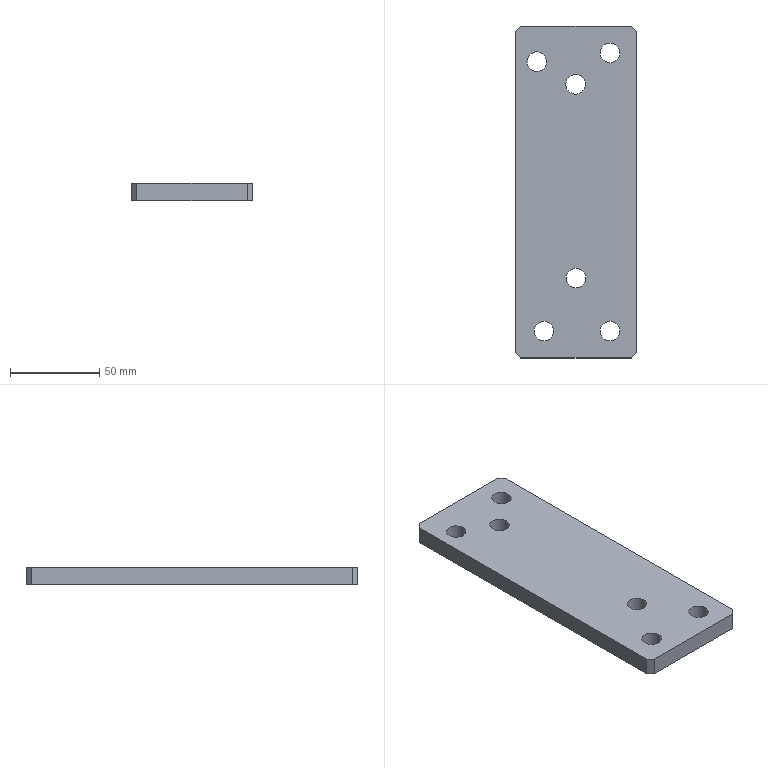Part | STEP file | 1_id206_x_t | 1 solid | 16 faces | box 68 x 186 x 10 mm | volume 120598 mm3 | plane 10 | cylinder 6 | commonest cylinder face diameters 11 x6
STEP:
#1=CARTESIAN_POINT('',(0.,0.,0.));
#2=DIRECTION('',(0.,0.,1.));
#3=DIRECTION('',(1.,0.,0.));
#4=AXIS2_PLACEMENT_3D('',#1,#2,#3);
#5=CARTESIAN_POINT('',(190.65,188.297,100.11));
#6=VERTEX_POINT('',#5);
#7=CARTESIAN_POINT('',(185.15,188.297,100.11));
#8=DIRECTION('',(0.,0.,-1.));
#9=DIRECTION('',(1.,0.,0.));
#10=AXIS2_PLACEMENT_3D('',#7,#8,#9);
#11=CIRCLE('',#10,5.5);
#12=CARTESIAN_POINT('',(185.15,188.297,-100.11));
#13=DIRECTION('',(0.,0.,1.));
#14=DIRECTION('',(1.,0.,0.));
#15=AXIS2_PLACEMENT_3D('',#12,#13,#14);
#16=CYLINDRICAL_SURFACE('',#15,5.5);
#17=CARTESIAN_POINT('',(6.283,200.22));
#18=DIRECTION('',(-1.,0.));
#19=VECTOR('',#18,1.);
#20=LINE('',#17,#19);
#21=(GEOMETRIC_REPRESENTATION_CONTEXT(2)PARAMETRIC_REPRESENTATION_CONTEXT()REPRESENTATION_CONTEXT('',''));
#22=DEFINITIONAL_REPRESENTATION('',(#20),#21);
#23=PCURVE('',#16,#22);
#24=CARTESIAN_POINT('',(239.613,193.297,100.11));
#25=DIRECTION('',(0.,0.,1.));
#26=DIRECTION('',(1.,0.,0.));
#27=AXIS2_PLACEMENT_3D('',#24,#25,#26);
#28=PLANE('',#27);
#29=CARTESIAN_POINT('',(-48.962,-5.));
#30=CARTESIAN_POINT('',(-48.962,-14.526));
#31=CARTESIAN_POINT('',(-57.212,-9.763));
#32=CARTESIAN_POINT('',(-65.463,-5.));
#33=CARTESIAN_POINT('',(-57.212,-0.2369));
#34=CARTESIAN_POINT('',(-48.962,4.526));
#35=CARTESIAN_POINT('',(-48.962,-5.));
#36=(BOUNDED_CURVE()B_SPLINE_CURVE(2,(#29,#30,#31,#32,#33,#34,#35),.UNSPECIFIED.,.T.,.F.)B_SPLINE_CURVE_WITH_KNOTS((1,2,2,2,2,1),(-2.094,0.,2.094,4.189,6.283,8.378),.UNSPECIFIED.)CURVE()GEOMETRIC_REPRESENTATION_ITEM()RATIONAL_B_SPLINE_CURVE((1.,0.5,1.,0.5,1.,0.5,1.))REPRESENTATION_ITEM(''));
#37=(GEOMETRIC_REPRESENTATION_CONTEXT(2)PARAMETRIC_REPRESENTATION_CONTEXT()REPRESENTATION_CONTEXT('',''));
#38=DEFINITIONAL_REPRESENTATION('',(#36),#37);
#39=PCURVE('',#28,#38);
#40=SURFACE_CURVE('',#11,(#23,#39),.PCURVE_S1.);
#41=EDGE_CURVE('',#6,#6,#40,.T.);
#42=ORIENTED_EDGE('',*,*,#41,.T.);
#43=CARTESIAN_POINT('',(190.65,188.297,90.11));
#44=VERTEX_POINT('',#43);
#45=CARTESIAN_POINT('',(190.65,188.297,90.11));
#46=CARTESIAN_POINT('',(190.65,188.297,100.11));
#47=B_SPLINE_CURVE_WITH_KNOTS('',1,(#45,#46),.UNSPECIFIED.,.F.,.F.,(2,2),(190.22,200.22),.PIECEWISE_BEZIER_KNOTS.);
#48=CARTESIAN_POINT('',(0.,0.));
#49=DIRECTION('',(0.,1.));
#50=VECTOR('',#49,1.);
#51=LINE('',#48,#50);
#52=(GEOMETRIC_REPRESENTATION_CONTEXT(2)PARAMETRIC_REPRESENTATION_CONTEXT()REPRESENTATION_CONTEXT('',''));
#53=DEFINITIONAL_REPRESENTATION('',(#51),#52);
#54=PCURVE('',#16,#53);
#55=CARTESIAN_POINT('',(6.283,0.));
#56=DIRECTION('',(0.,1.));
#57=VECTOR('',#56,1.);
#58=LINE('',#55,#57);
#59=(GEOMETRIC_REPRESENTATION_CONTEXT(2)PARAMETRIC_REPRESENTATION_CONTEXT()REPRESENTATION_CONTEXT('',''));
#60=DEFINITIONAL_REPRESENTATION('',(#58),#59);
#61=PCURVE('',#16,#60);
#62=SEAM_CURVE('',#47,(#54,#61),.PCURVE_S1.);
#63=EDGE_CURVE('',#44,#6,#62,.T.);
#64=ORIENTED_EDGE('',*,*,#63,.F.);
#65=CARTESIAN_POINT('',(185.15,188.297,90.11));
#66=DIRECTION('',(0.,0.,-1.));
#67=DIRECTION('',(1.,0.,0.));
#68=AXIS2_PLACEMENT_3D('',#65,#66,#67);
#69=CIRCLE('',#68,5.5);
#70=CARTESIAN_POINT('',(6.283,190.22));
#71=DIRECTION('',(-1.,0.));
#72=VECTOR('',#71,1.);
#73=LINE('',#70,#72);
#74=(GEOMETRIC_REPRESENTATION_CONTEXT(2)PARAMETRIC_REPRESENTATION_CONTEXT()REPRESENTATION_CONTEXT('',''));
#75=DEFINITIONAL_REPRESENTATION('',(#73),#74);
#76=PCURVE('',#16,#75);
#77=CARTESIAN_POINT('',(244.613,193.297,90.11));
#78=DIRECTION('',(0.,0.,1.));
#79=DIRECTION('',(1.,0.,0.));
#80=AXIS2_PLACEMENT_3D('',#77,#78,#79);
#81=PLANE('',#80);
#82=CARTESIAN_POINT('',(-53.962,-5.));
#83=CARTESIAN_POINT('',(-53.962,-14.526));
#84=CARTESIAN_POINT('',(-62.212,-9.763));
#85=CARTESIAN_POINT('',(-70.463,-5.));
#86=CARTESIAN_POINT('',(-62.212,-0.2369));
#87=CARTESIAN_POINT('',(-53.962,4.526));
#88=CARTESIAN_POINT('',(-53.962,-5.));
#89=(BOUNDED_CURVE()B_SPLINE_CURVE(2,(#82,#83,#84,#85,#86,#87,#88),.UNSPECIFIED.,.T.,.F.)B_SPLINE_CURVE_WITH_KNOTS((1,2,2,2,2,1),(-2.094,0.,2.094,4.189,6.283,8.378),.UNSPECIFIED.)CURVE()GEOMETRIC_REPRESENTATION_ITEM()RATIONAL_B_SPLINE_CURVE((1.,0.5,1.,0.5,1.,0.5,1.))REPRESENTATION_ITEM(''));
#90=(GEOMETRIC_REPRESENTATION_CONTEXT(2)PARAMETRIC_REPRESENTATION_CONTEXT()REPRESENTATION_CONTEXT('',''));
#91=DEFINITIONAL_REPRESENTATION('',(#89),#90);
#92=PCURVE('',#81,#91);
#93=SURFACE_CURVE('',#69,(#76,#92),.PCURVE_S1.);
#94=EDGE_CURVE('',#44,#44,#93,.T.);
#95=ORIENTED_EDGE('',*,*,#94,.F.);
#96=ORIENTED_EDGE('',*,*,#63,.T.);
#97=EDGE_LOOP('',(#42,#64,#95,#96));
#98=FACE_BOUND('',#97,.F.);
#99=ADVANCED_FACE('',(#98),#16,.F.);
#100=CARTESIAN_POINT('',(238.15,208.297,90.11));
#101=VERTEX_POINT('',#100);
#102=CARTESIAN_POINT('',(238.15,208.297,100.11));
#103=VERTEX_POINT('',#102);
#104=CARTESIAN_POINT('',(238.15,208.297,90.11));
#105=DIRECTION('',(0.,0.,1.));
#106=VECTOR('',#105,1.);
#107=LINE('',#104,#106);
#108=CARTESIAN_POINT('',(238.881,207.565,100.11));
#109=DIRECTION('',(-0.7071,-0.7071,0.));
#110=DIRECTION('',(-0.7071,0.7071,0.));
#111=AXIS2_PLACEMENT_3D('',#108,#109,#110);
#112=PLANE('',#111);
#113=CARTESIAN_POINT('',(1.034,10.));
#114=DIRECTION('',(0.,-1.));
#115=VECTOR('',#114,1.);
#116=LINE('',#113,#115);
#117=(GEOMETRIC_REPRESENTATION_CONTEXT(2)PARAMETRIC_REPRESENTATION_CONTEXT()REPRESENTATION_CONTEXT('',''));
#118=DEFINITIONAL_REPRESENTATION('',(#116),#117);
#119=PCURVE('',#112,#118);
#120=CARTESIAN_POINT('',(174.688,208.297,100.11));
#121=DIRECTION('',(0.,-1.,0.));
#122=DIRECTION('',(0.,0.,-1.));
#123=AXIS2_PLACEMENT_3D('',#120,#121,#122);
#124=PLANE('',#123);
#125=CARTESIAN_POINT('',(10.,63.462));
#126=DIRECTION('',(-1.,0.));
#127=VECTOR('',#126,1.);
#128=LINE('',#125,#127);
#129=(GEOMETRIC_REPRESENTATION_CONTEXT(2)PARAMETRIC_REPRESENTATION_CONTEXT()REPRESENTATION_CONTEXT('',''));
#130=DEFINITIONAL_REPRESENTATION('',(#128),#129);
#131=PCURVE('',#124,#130);
#132=SURFACE_CURVE('',#107,(#119,#131),.PCURVE_S1.);
#133=EDGE_CURVE('',#101,#103,#132,.T.);
#134=ORIENTED_EDGE('',*,*,#133,.T.);
#135=CARTESIAN_POINT('',(241.15,205.297,100.11));
#136=VERTEX_POINT('',#135);
#137=CARTESIAN_POINT('',(241.15,205.297,100.11));
#138=DIRECTION('',(-0.7071,0.7071,0.));
#139=VECTOR('',#138,1.);
#140=LINE('',#137,#139);
#141=CARTESIAN_POINT('',(-3.208,0.));
#142=DIRECTION('',(1.,0.));
#143=VECTOR('',#142,1.);
#144=LINE('',#141,#143);
#145=(GEOMETRIC_REPRESENTATION_CONTEXT(2)PARAMETRIC_REPRESENTATION_CONTEXT()REPRESENTATION_CONTEXT('',''));
#146=DEFINITIONAL_REPRESENTATION('',(#144),#145);
#147=PCURVE('',#112,#146);
#148=CARTESIAN_POINT('',(1.538,12.));
#149=DIRECTION('',(-0.7071,0.7071));
#150=VECTOR('',#149,1.);
#151=LINE('',#148,#150);
#152=(GEOMETRIC_REPRESENTATION_CONTEXT(2)PARAMETRIC_REPRESENTATION_CONTEXT()REPRESENTATION_CONTEXT('',''));
#153=DEFINITIONAL_REPRESENTATION('',(#151),#152);
#154=PCURVE('',#28,#153);
#155=SURFACE_CURVE('',#140,(#147,#154),.PCURVE_S1.);
#156=EDGE_CURVE('',#136,#103,#155,.T.);
#157=ORIENTED_EDGE('',*,*,#156,.F.);
#158=CARTESIAN_POINT('',(241.15,205.297,90.11));
#159=VERTEX_POINT('',#158);
#160=CARTESIAN_POINT('',(241.15,205.297,90.11));
#161=DIRECTION('',(0.,0.,1.));
#162=VECTOR('',#161,1.);
#163=LINE('',#160,#162);
#164=CARTESIAN_POINT('',(-3.208,10.));
#165=DIRECTION('',(0.,-1.));
#166=VECTOR('',#165,1.);
#167=LINE('',#164,#166);
#168=(GEOMETRIC_REPRESENTATION_CONTEXT(2)PARAMETRIC_REPRESENTATION_CONTEXT()REPRESENTATION_CONTEXT('',''));
#169=DEFINITIONAL_REPRESENTATION('',(#167),#168);
#170=PCURVE('',#112,#169);
#171=CARTESIAN_POINT('',(241.15,38.297,100.11));
#172=DIRECTION('',(-1.,0.,0.));
#173=DIRECTION('',(0.,1.,0.));
#174=AXIS2_PLACEMENT_3D('',#171,#172,#173);
#175=PLANE('',#174);
#176=CARTESIAN_POINT('',(167.,10.));
#177=DIRECTION('',(0.,-1.));
#178=VECTOR('',#177,1.);
#179=LINE('',#176,#178);
#180=(GEOMETRIC_REPRESENTATION_CONTEXT(2)PARAMETRIC_REPRESENTATION_CONTEXT()REPRESENTATION_CONTEXT('',''));
#181=DEFINITIONAL_REPRESENTATION('',(#179),#180);
#182=PCURVE('',#175,#181);
#183=SURFACE_CURVE('',#163,(#170,#182),.PCURVE_S1.);
#184=EDGE_CURVE('',#159,#136,#183,.T.);
#185=ORIENTED_EDGE('',*,*,#184,.F.);
#186=CARTESIAN_POINT('',(238.15,208.297,90.11));
#187=DIRECTION('',(0.7071,-0.7071,0.));
#188=VECTOR('',#187,1.);
#189=LINE('',#186,#188);
#190=CARTESIAN_POINT('',(1.034,10.));
#191=DIRECTION('',(-1.,0.));
#192=VECTOR('',#191,1.);
#193=LINE('',#190,#192);
#194=(GEOMETRIC_REPRESENTATION_CONTEXT(2)PARAMETRIC_REPRESENTATION_CONTEXT()REPRESENTATION_CONTEXT('',''));
#195=DEFINITIONAL_REPRESENTATION('',(#193),#194);
#196=PCURVE('',#112,#195);
#197=CARTESIAN_POINT('',(-6.463,15.));
#198=DIRECTION('',(0.7071,-0.7071));
#199=VECTOR('',#198,1.);
#200=LINE('',#197,#199);
#201=(GEOMETRIC_REPRESENTATION_CONTEXT(2)PARAMETRIC_REPRESENTATION_CONTEXT()REPRESENTATION_CONTEXT('',''));
#202=DEFINITIONAL_REPRESENTATION('',(#200),#201);
#203=PCURVE('',#81,#202);
#204=SURFACE_CURVE('',#189,(#196,#203),.PCURVE_S1.);
#205=EDGE_CURVE('',#101,#159,#204,.T.);
#206=ORIENTED_EDGE('',*,*,#205,.F.);
#207=EDGE_LOOP('',(#134,#157,#185,#206));
#208=FACE_BOUND('',#207,.T.);
#209=ADVANCED_FACE('',(#208),#112,.F.);
#210=CARTESIAN_POINT('',(176.15,208.297,90.11));
#211=VERTEX_POINT('',#210);
#212=CARTESIAN_POINT('',(176.15,208.297,100.11));
#213=VERTEX_POINT('',#212);
#214=CARTESIAN_POINT('',(176.15,208.297,90.11));
#215=DIRECTION('',(0.,0.,1.));
#216=VECTOR('',#215,1.);
#217=LINE('',#214,#216);
#218=CARTESIAN_POINT('',(10.,1.462));
#219=DIRECTION('',(-1.,0.));
#220=VECTOR('',#219,1.);
#221=LINE('',#218,#220);
#222=(GEOMETRIC_REPRESENTATION_CONTEXT(2)PARAMETRIC_REPRESENTATION_CONTEXT()REPRESENTATION_CONTEXT('',''));
#223=DEFINITIONAL_REPRESENTATION('',(#221),#222);
#224=PCURVE('',#124,#223);
#225=CARTESIAN_POINT('',(207.881,240.028,100.11));
#226=DIRECTION('',(0.7071,-0.7071,0.));
#227=DIRECTION('',(-0.7071,-0.7071,0.));
#228=AXIS2_PLACEMENT_3D('',#225,#226,#227);
#229=PLANE('',#228);
#230=CARTESIAN_POINT('',(44.875,10.));
#231=DIRECTION('',(0.,-1.));
#232=VECTOR('',#231,1.);
#233=LINE('',#230,#232);
#234=(GEOMETRIC_REPRESENTATION_CONTEXT(2)PARAMETRIC_REPRESENTATION_CONTEXT()REPRESENTATION_CONTEXT('',''));
#235=DEFINITIONAL_REPRESENTATION('',(#233),#234);
#236=PCURVE('',#229,#235);
#237=SURFACE_CURVE('',#217,(#224,#236),.PCURVE_S1.);
#238=EDGE_CURVE('',#211,#213,#237,.T.);
#239=ORIENTED_EDGE('',*,*,#238,.T.);
#240=CARTESIAN_POINT('',(238.15,208.297,100.11));
#241=DIRECTION('',(-1.,0.,0.));
#242=VECTOR('',#241,1.);
#243=LINE('',#240,#242);
#244=CARTESIAN_POINT('',(0.,63.462));
#245=DIRECTION('',(0.,-1.));
#246=VECTOR('',#245,1.);
#247=LINE('',#244,#246);
#248=(GEOMETRIC_REPRESENTATION_CONTEXT(2)PARAMETRIC_REPRESENTATION_CONTEXT()REPRESENTATION_CONTEXT('',''));
#249=DEFINITIONAL_REPRESENTATION('',(#247),#248);
#250=PCURVE('',#124,#249);
#251=CARTESIAN_POINT('',(-1.462,15.));
#252=DIRECTION('',(-1.,0.));
#253=VECTOR('',#252,1.);
#254=LINE('',#251,#253);
#255=(GEOMETRIC_REPRESENTATION_CONTEXT(2)PARAMETRIC_REPRESENTATION_CONTEXT()REPRESENTATION_CONTEXT('',''));
#256=DEFINITIONAL_REPRESENTATION('',(#254),#255);
#257=PCURVE('',#28,#256);
#258=SURFACE_CURVE('',#243,(#250,#257),.PCURVE_S1.);
#259=EDGE_CURVE('',#103,#213,#258,.T.);
#260=ORIENTED_EDGE('',*,*,#259,.F.);
#261=ORIENTED_EDGE('',*,*,#133,.F.);
#262=CARTESIAN_POINT('',(238.15,208.297,90.11));
#263=DIRECTION('',(-1.,0.,0.));
#264=VECTOR('',#263,1.);
#265=LINE('',#262,#264);
#266=CARTESIAN_POINT('',(10.,63.462));
#267=DIRECTION('',(0.,-1.));
#268=VECTOR('',#267,1.);
#269=LINE('',#266,#268);
#270=(GEOMETRIC_REPRESENTATION_CONTEXT(2)PARAMETRIC_REPRESENTATION_CONTEXT()REPRESENTATION_CONTEXT('',''));
#271=DEFINITIONAL_REPRESENTATION('',(#269),#270);
#272=PCURVE('',#124,#271);
#273=CARTESIAN_POINT('',(-6.463,15.));
#274=DIRECTION('',(-1.,0.));
#275=VECTOR('',#274,1.);
#276=LINE('',#273,#275);
#277=(GEOMETRIC_REPRESENTATION_CONTEXT(2)PARAMETRIC_REPRESENTATION_CONTEXT()REPRESENTATION_CONTEXT('',''));
#278=DEFINITIONAL_REPRESENTATION('',(#276),#277);
#279=PCURVE('',#81,#278);
#280=SURFACE_CURVE('',#265,(#272,#279),.PCURVE_S1.);
#281=EDGE_CURVE('',#101,#211,#280,.T.);
#282=ORIENTED_EDGE('',*,*,#281,.T.);
#283=EDGE_LOOP('',(#239,#260,#261,#282));
#284=FACE_BOUND('',#283,.T.);
#285=ADVANCED_FACE('',(#284),#124,.F.);
#286=CARTESIAN_POINT('',(173.15,205.297,90.11));
#287=VERTEX_POINT('',#286);
#288=CARTESIAN_POINT('',(173.15,205.297,100.11));
#289=VERTEX_POINT('',#288);
#290=CARTESIAN_POINT('',(173.15,205.297,90.11));
#291=DIRECTION('',(0.,0.,1.));
#292=VECTOR('',#291,1.);
#293=LINE('',#290,#292);
#294=CARTESIAN_POINT('',(49.117,10.));
#295=DIRECTION('',(0.,-1.));
#296=VECTOR('',#295,1.);
#297=LINE('',#294,#296);
#298=(GEOMETRIC_REPRESENTATION_CONTEXT(2)PARAMETRIC_REPRESENTATION_CONTEXT()REPRESENTATION_CONTEXT('',''));
#299=DEFINITIONAL_REPRESENTATION('',(#297),#298);
#300=PCURVE('',#229,#299);
#301=CARTESIAN_POINT('',(173.15,38.297,100.11));
#302=DIRECTION('',(1.,0.,0.));
#303=DIRECTION('',(0.,-1.,0.));
#304=AXIS2_PLACEMENT_3D('',#301,#302,#303);
#305=PLANE('',#304);
#306=CARTESIAN_POINT('',(-167.,10.));
#307=DIRECTION('',(0.,-1.));
#308=VECTOR('',#307,1.);
#309=LINE('',#306,#308);
#310=(GEOMETRIC_REPRESENTATION_CONTEXT(2)PARAMETRIC_REPRESENTATION_CONTEXT()REPRESENTATION_CONTEXT('',''));
#311=DEFINITIONAL_REPRESENTATION('',(#309),#310);
#312=PCURVE('',#305,#311);
#313=SURFACE_CURVE('',#293,(#300,#312),.PCURVE_S1.);
#314=EDGE_CURVE('',#287,#289,#313,.T.);
#315=ORIENTED_EDGE('',*,*,#314,.T.);
#316=CARTESIAN_POINT('',(176.15,208.297,100.11));
#317=DIRECTION('',(-0.7071,-0.7071,0.));
#318=VECTOR('',#317,1.);
#319=LINE('',#316,#318);
#320=CARTESIAN_POINT('',(44.875,0.));
#321=DIRECTION('',(1.,0.));
#322=VECTOR('',#321,1.);
#323=LINE('',#320,#322);
#324=(GEOMETRIC_REPRESENTATION_CONTEXT(2)PARAMETRIC_REPRESENTATION_CONTEXT()REPRESENTATION_CONTEXT('',''));
#325=DEFINITIONAL_REPRESENTATION('',(#323),#324);
#326=PCURVE('',#229,#325);
#327=CARTESIAN_POINT('',(-63.462,15.));
#328=DIRECTION('',(-0.7071,-0.7071));
#329=VECTOR('',#328,1.);
#330=LINE('',#327,#329);
#331=(GEOMETRIC_REPRESENTATION_CONTEXT(2)PARAMETRIC_REPRESENTATION_CONTEXT()REPRESENTATION_CONTEXT('',''));
#332=DEFINITIONAL_REPRESENTATION('',(#330),#331);
#333=PCURVE('',#28,#332);
#334=SURFACE_CURVE('',#319,(#326,#333),.PCURVE_S1.);
#335=EDGE_CURVE('',#213,#289,#334,.T.);
#336=ORIENTED_EDGE('',*,*,#335,.F.);
#337=ORIENTED_EDGE('',*,*,#238,.F.);
#338=CARTESIAN_POINT('',(173.15,205.297,90.11));
#339=DIRECTION('',(0.7071,0.7071,0.));
#340=VECTOR('',#339,1.);
#341=LINE('',#338,#340);
#342=CARTESIAN_POINT('',(49.117,10.));
#343=DIRECTION('',(-1.,0.));
#344=VECTOR('',#343,1.);
#345=LINE('',#342,#344);
#346=(GEOMETRIC_REPRESENTATION_CONTEXT(2)PARAMETRIC_REPRESENTATION_CONTEXT()REPRESENTATION_CONTEXT('',''));
#347=DEFINITIONAL_REPRESENTATION('',(#345),#346);
#348=PCURVE('',#229,#347);
#349=CARTESIAN_POINT('',(-71.463,12.));
#350=DIRECTION('',(0.7071,0.7071));
#351=VECTOR('',#350,1.);
#352=LINE('',#349,#351);
#353=(GEOMETRIC_REPRESENTATION_CONTEXT(2)PARAMETRIC_REPRESENTATION_CONTEXT()REPRESENTATION_CONTEXT('',''));
#354=DEFINITIONAL_REPRESENTATION('',(#352),#353);
#355=PCURVE('',#81,#354);
#356=SURFACE_CURVE('',#341,(#348,#355),.PCURVE_S1.);
#357=EDGE_CURVE('',#287,#211,#356,.T.);
#358=ORIENTED_EDGE('',*,*,#357,.F.);
#359=EDGE_LOOP('',(#315,#336,#337,#358));
#360=FACE_BOUND('',#359,.T.);
#361=ADVANCED_FACE('',(#360),#229,.F.);
#362=ORIENTED_EDGE('',*,*,#314,.F.);
#363=CARTESIAN_POINT('',(173.15,25.297,90.11));
#364=VERTEX_POINT('',#363);
#365=CARTESIAN_POINT('',(173.15,205.297,90.11));
#366=DIRECTION('',(0.,-1.,0.));
#367=VECTOR('',#366,1.);
#368=LINE('',#365,#367);
#369=CARTESIAN_POINT('',(-167.,10.));
#370=DIRECTION('',(1.,0.));
#371=VECTOR('',#370,1.);
#372=LINE('',#369,#371);
#373=(GEOMETRIC_REPRESENTATION_CONTEXT(2)PARAMETRIC_REPRESENTATION_CONTEXT()REPRESENTATION_CONTEXT('',''));
#374=DEFINITIONAL_REPRESENTATION('',(#372),#373);
#375=PCURVE('',#305,#374);
#376=CARTESIAN_POINT('',(-71.463,12.));
#377=DIRECTION('',(0.,-1.));
#378=VECTOR('',#377,1.);
#379=LINE('',#376,#378);
#380=(GEOMETRIC_REPRESENTATION_CONTEXT(2)PARAMETRIC_REPRESENTATION_CONTEXT()REPRESENTATION_CONTEXT('',''));
#381=DEFINITIONAL_REPRESENTATION('',(#379),#380);
#382=PCURVE('',#81,#381);
#383=SURFACE_CURVE('',#368,(#375,#382),.PCURVE_S1.);
#384=EDGE_CURVE('',#287,#364,#383,.T.);
#385=ORIENTED_EDGE('',*,*,#384,.T.);
#386=CARTESIAN_POINT('',(173.15,25.297,100.11));
#387=VERTEX_POINT('',#386);
#388=CARTESIAN_POINT('',(173.15,25.297,90.11));
#389=DIRECTION('',(0.,0.,1.));
#390=VECTOR('',#389,1.);
#391=LINE('',#388,#390);
#392=CARTESIAN_POINT('',(13.,10.));
#393=DIRECTION('',(0.,-1.));
#394=VECTOR('',#393,1.);
#395=LINE('',#392,#394);
#396=(GEOMETRIC_REPRESENTATION_CONTEXT(2)PARAMETRIC_REPRESENTATION_CONTEXT()REPRESENTATION_CONTEXT('',''));
#397=DEFINITIONAL_REPRESENTATION('',(#395),#396);
#398=PCURVE('',#305,#397);
#399=CARTESIAN_POINT('',(130.381,68.065,100.11));
#400=DIRECTION('',(0.7071,0.7071,0.));
#401=DIRECTION('',(0.7071,-0.7071,0.));
#402=AXIS2_PLACEMENT_3D('',#399,#400,#401);
#403=PLANE('',#402);
#404=CARTESIAN_POINT('',(60.484,10.));
#405=DIRECTION('',(0.,-1.));
#406=VECTOR('',#405,1.);
#407=LINE('',#404,#406);
#408=(GEOMETRIC_REPRESENTATION_CONTEXT(2)PARAMETRIC_REPRESENTATION_CONTEXT()REPRESENTATION_CONTEXT('',''));
#409=DEFINITIONAL_REPRESENTATION('',(#407),#408);
#410=PCURVE('',#403,#409);
#411=SURFACE_CURVE('',#391,(#398,#410),.PCURVE_S1.);
#412=EDGE_CURVE('',#364,#387,#411,.T.);
#413=ORIENTED_EDGE('',*,*,#412,.T.);
#414=CARTESIAN_POINT('',(173.15,205.297,100.11));
#415=DIRECTION('',(0.,-1.,0.));
#416=VECTOR('',#415,1.);
#417=LINE('',#414,#416);
#418=CARTESIAN_POINT('',(-167.,0.));
#419=DIRECTION('',(1.,0.));
#420=VECTOR('',#419,1.);
#421=LINE('',#418,#420);
#422=(GEOMETRIC_REPRESENTATION_CONTEXT(2)PARAMETRIC_REPRESENTATION_CONTEXT()REPRESENTATION_CONTEXT('',''));
#423=DEFINITIONAL_REPRESENTATION('',(#421),#422);
#424=PCURVE('',#305,#423);
#425=CARTESIAN_POINT('',(-66.463,12.));
#426=DIRECTION('',(0.,-1.));
#427=VECTOR('',#426,1.);
#428=LINE('',#425,#427);
#429=(GEOMETRIC_REPRESENTATION_CONTEXT(2)PARAMETRIC_REPRESENTATION_CONTEXT()REPRESENTATION_CONTEXT('',''));
#430=DEFINITIONAL_REPRESENTATION('',(#428),#429);
#431=PCURVE('',#28,#430);
#432=SURFACE_CURVE('',#417,(#424,#431),.PCURVE_S1.);
#433=EDGE_CURVE('',#289,#387,#432,.T.);
#434=ORIENTED_EDGE('',*,*,#433,.F.);
#435=EDGE_LOOP('',(#362,#385,#413,#434));
#436=FACE_BOUND('',#435,.T.);
#437=ADVANCED_FACE('',(#436),#305,.F.);
#438=CARTESIAN_POINT('',(176.15,22.297,90.11));
#439=VERTEX_POINT('',#438);
#440=CARTESIAN_POINT('',(176.15,22.297,100.11));
#441=VERTEX_POINT('',#440);
#442=CARTESIAN_POINT('',(176.15,22.297,90.11));
#443=DIRECTION('',(0.,0.,1.));
#444=VECTOR('',#443,1.);
#445=LINE('',#442,#444);
#446=CARTESIAN_POINT('',(64.727,10.));
#447=DIRECTION('',(0.,-1.));
#448=VECTOR('',#447,1.);
#449=LINE('',#446,#448);
#450=(GEOMETRIC_REPRESENTATION_CONTEXT(2)PARAMETRIC_REPRESENTATION_CONTEXT()REPRESENTATION_CONTEXT('',''));
#451=DEFINITIONAL_REPRESENTATION('',(#449),#450);
#452=PCURVE('',#403,#451);
#453=CARTESIAN_POINT('',(239.613,22.297,100.11));
#454=DIRECTION('',(0.,1.,0.));
#455=DIRECTION('',(0.,0.,1.));
#456=AXIS2_PLACEMENT_3D('',#453,#454,#455);
#457=PLANE('',#456);
#458=CARTESIAN_POINT('',(-10.,-63.462));
#459=DIRECTION('',(1.,0.));
#460=VECTOR('',#459,1.);
#461=LINE('',#458,#460);
#462=(GEOMETRIC_REPRESENTATION_CONTEXT(2)PARAMETRIC_REPRESENTATION_CONTEXT()REPRESENTATION_CONTEXT('',''));
#463=DEFINITIONAL_REPRESENTATION('',(#461),#462);
#464=PCURVE('',#457,#463);
#465=SURFACE_CURVE('',#445,(#452,#464),.PCURVE_S1.);
#466=EDGE_CURVE('',#439,#441,#465,.T.);
#467=ORIENTED_EDGE('',*,*,#466,.T.);
#468=CARTESIAN_POINT('',(173.15,25.297,100.11));
#469=DIRECTION('',(0.7071,-0.7071,0.));
#470=VECTOR('',#469,1.);
#471=LINE('',#468,#470);
#472=CARTESIAN_POINT('',(60.484,0.));
#473=DIRECTION('',(1.,0.));
#474=VECTOR('',#473,1.);
#475=LINE('',#472,#474);
#476=(GEOMETRIC_REPRESENTATION_CONTEXT(2)PARAMETRIC_REPRESENTATION_CONTEXT()REPRESENTATION_CONTEXT('',''));
#477=DEFINITIONAL_REPRESENTATION('',(#475),#476);
#478=PCURVE('',#403,#477);
#479=CARTESIAN_POINT('',(-66.463,-168.));
#480=DIRECTION('',(0.7071,-0.7071));
#481=VECTOR('',#480,1.);
#482=LINE('',#479,#481);
#483=(GEOMETRIC_REPRESENTATION_CONTEXT(2)PARAMETRIC_REPRESENTATION_CONTEXT()REPRESENTATION_CONTEXT('',''));
#484=DEFINITIONAL_REPRESENTATION('',(#482),#483);
#485=PCURVE('',#28,#484);
#486=SURFACE_CURVE('',#471,(#478,#485),.PCURVE_S1.);
#487=EDGE_CURVE('',#387,#441,#486,.T.);
#488=ORIENTED_EDGE('',*,*,#487,.F.);
#489=ORIENTED_EDGE('',*,*,#412,.F.);
#490=CARTESIAN_POINT('',(176.15,22.297,90.11));
#491=DIRECTION('',(-0.7071,0.7071,0.));
#492=VECTOR('',#491,1.);
#493=LINE('',#490,#492);
#494=CARTESIAN_POINT('',(64.727,10.));
#495=DIRECTION('',(-1.,0.));
#496=VECTOR('',#495,1.);
#497=LINE('',#494,#496);
#498=(GEOMETRIC_REPRESENTATION_CONTEXT(2)PARAMETRIC_REPRESENTATION_CONTEXT()REPRESENTATION_CONTEXT('',''));
#499=DEFINITIONAL_REPRESENTATION('',(#497),#498);
#500=PCURVE('',#403,#499);
#501=CARTESIAN_POINT('',(-68.463,-171.));
#502=DIRECTION('',(-0.7071,0.7071));
#503=VECTOR('',#502,1.);
#504=LINE('',#501,#503);
#505=(GEOMETRIC_REPRESENTATION_CONTEXT(2)PARAMETRIC_REPRESENTATION_CONTEXT()REPRESENTATION_CONTEXT('',''));
#506=DEFINITIONAL_REPRESENTATION('',(#504),#505);
#507=PCURVE('',#81,#506);
#508=SURFACE_CURVE('',#493,(#500,#507),.PCURVE_S1.);
#509=EDGE_CURVE('',#439,#364,#508,.T.);
#510=ORIENTED_EDGE('',*,*,#509,.F.);
#511=EDGE_LOOP('',(#467,#488,#489,#510));
#512=FACE_BOUND('',#511,.T.);
#513=ADVANCED_FACE('',(#512),#403,.F.);
#514=CARTESIAN_POINT('',(238.15,22.297,90.11));
#515=VERTEX_POINT('',#514);
#516=CARTESIAN_POINT('',(238.15,22.297,100.11));
#517=VERTEX_POINT('',#516);
#518=CARTESIAN_POINT('',(238.15,22.297,90.11));
#519=DIRECTION('',(0.,0.,1.));
#520=VECTOR('',#519,1.);
#521=LINE('',#518,#520);
#522=CARTESIAN_POINT('',(-10.,-1.462));
#523=DIRECTION('',(1.,0.));
#524=VECTOR('',#523,1.);
#525=LINE('',#522,#524);
#526=(GEOMETRIC_REPRESENTATION_CONTEXT(2)PARAMETRIC_REPRESENTATION_CONTEXT()REPRESENTATION_CONTEXT('',''));
#527=DEFINITIONAL_REPRESENTATION('',(#525),#526);
#528=PCURVE('',#457,#527);
#529=CARTESIAN_POINT('',(316.381,100.528,100.11));
#530=DIRECTION('',(-0.7071,0.7071,0.));
#531=DIRECTION('',(0.7071,0.7071,0.));
#532=AXIS2_PLACEMENT_3D('',#529,#530,#531);
#533=PLANE('',#532);
#534=CARTESIAN_POINT('',(-110.636,10.));
#535=DIRECTION('',(0.,-1.));
#536=VECTOR('',#535,1.);
#537=LINE('',#534,#536);
#538=(GEOMETRIC_REPRESENTATION_CONTEXT(2)PARAMETRIC_REPRESENTATION_CONTEXT()REPRESENTATION_CONTEXT('',''));
#539=DEFINITIONAL_REPRESENTATION('',(#537),#538);
#540=PCURVE('',#533,#539);
#541=SURFACE_CURVE('',#521,(#528,#540),.PCURVE_S1.);
#542=EDGE_CURVE('',#515,#517,#541,.T.);
#543=ORIENTED_EDGE('',*,*,#542,.T.);
#544=CARTESIAN_POINT('',(176.15,22.297,100.11));
#545=DIRECTION('',(1.,0.,0.));
#546=VECTOR('',#545,1.);
#547=LINE('',#544,#546);
#548=CARTESIAN_POINT('',(0.,-63.462));
#549=DIRECTION('',(0.,1.));
#550=VECTOR('',#549,1.);
#551=LINE('',#548,#550);
#552=(GEOMETRIC_REPRESENTATION_CONTEXT(2)PARAMETRIC_REPRESENTATION_CONTEXT()REPRESENTATION_CONTEXT('',''));
#553=DEFINITIONAL_REPRESENTATION('',(#551),#552);
#554=PCURVE('',#457,#553);
#555=CARTESIAN_POINT('',(-63.462,-171.));
#556=DIRECTION('',(1.,0.));
#557=VECTOR('',#556,1.);
#558=LINE('',#555,#557);
#559=(GEOMETRIC_REPRESENTATION_CONTEXT(2)PARAMETRIC_REPRESENTATION_CONTEXT()REPRESENTATION_CONTEXT('',''));
#560=DEFINITIONAL_REPRESENTATION('',(#558),#559);
#561=PCURVE('',#28,#560);
#562=SURFACE_CURVE('',#547,(#554,#561),.PCURVE_S1.);
#563=EDGE_CURVE('',#441,#517,#562,.T.);
#564=ORIENTED_EDGE('',*,*,#563,.F.);
#565=ORIENTED_EDGE('',*,*,#466,.F.);
#566=CARTESIAN_POINT('',(176.15,22.297,90.11));
#567=DIRECTION('',(1.,0.,0.));
#568=VECTOR('',#567,1.);
#569=LINE('',#566,#568);
#570=CARTESIAN_POINT('',(-10.,-63.462));
#571=DIRECTION('',(0.,1.));
#572=VECTOR('',#571,1.);
#573=LINE('',#570,#572);
#574=(GEOMETRIC_REPRESENTATION_CONTEXT(2)PARAMETRIC_REPRESENTATION_CONTEXT()REPRESENTATION_CONTEXT('',''));
#575=DEFINITIONAL_REPRESENTATION('',(#573),#574);
#576=PCURVE('',#457,#575);
#577=CARTESIAN_POINT('',(-68.463,-171.));
#578=DIRECTION('',(1.,0.));
#579=VECTOR('',#578,1.);
#580=LINE('',#577,#579);
#581=(GEOMETRIC_REPRESENTATION_CONTEXT(2)PARAMETRIC_REPRESENTATION_CONTEXT()REPRESENTATION_CONTEXT('',''));
#582=DEFINITIONAL_REPRESENTATION('',(#580),#581);
#583=PCURVE('',#81,#582);
#584=SURFACE_CURVE('',#569,(#576,#583),.PCURVE_S1.);
#585=EDGE_CURVE('',#439,#515,#584,.T.);
#586=ORIENTED_EDGE('',*,*,#585,.T.);
#587=EDGE_LOOP('',(#543,#564,#565,#586));
#588=FACE_BOUND('',#587,.T.);
#589=ADVANCED_FACE('',(#588),#457,.F.);
#590=CARTESIAN_POINT('',(241.15,25.297,90.11));
#591=VERTEX_POINT('',#590);
#592=CARTESIAN_POINT('',(241.15,25.297,100.11));
#593=VERTEX_POINT('',#592);
#594=CARTESIAN_POINT('',(241.15,25.297,90.11));
#595=DIRECTION('',(0.,0.,1.));
#596=VECTOR('',#595,1.);
#597=LINE('',#594,#596);
#598=CARTESIAN_POINT('',(-106.393,10.));
#599=DIRECTION('',(0.,-1.));
#600=VECTOR('',#599,1.);
#601=LINE('',#598,#600);
#602=(GEOMETRIC_REPRESENTATION_CONTEXT(2)PARAMETRIC_REPRESENTATION_CONTEXT()REPRESENTATION_CONTEXT('',''));
#603=DEFINITIONAL_REPRESENTATION('',(#601),#602);
#604=PCURVE('',#533,#603);
#605=CARTESIAN_POINT('',(-13.,10.));
#606=DIRECTION('',(0.,-1.));
#607=VECTOR('',#606,1.);
#608=LINE('',#605,#607);
#609=(GEOMETRIC_REPRESENTATION_CONTEXT(2)PARAMETRIC_REPRESENTATION_CONTEXT()REPRESENTATION_CONTEXT('',''));
#610=DEFINITIONAL_REPRESENTATION('',(#608),#609);
#611=PCURVE('',#175,#610);
#612=SURFACE_CURVE('',#597,(#604,#611),.PCURVE_S1.);
#613=EDGE_CURVE('',#591,#593,#612,.T.);
#614=ORIENTED_EDGE('',*,*,#613,.T.);
#615=CARTESIAN_POINT('',(238.15,22.297,100.11));
#616=DIRECTION('',(0.7071,0.7071,0.));
#617=VECTOR('',#616,1.);
#618=LINE('',#615,#617);
#619=CARTESIAN_POINT('',(-110.636,0.));
#620=DIRECTION('',(1.,0.));
#621=VECTOR('',#620,1.);
#622=LINE('',#619,#621);
#623=(GEOMETRIC_REPRESENTATION_CONTEXT(2)PARAMETRIC_REPRESENTATION_CONTEXT()REPRESENTATION_CONTEXT('',''));
#624=DEFINITIONAL_REPRESENTATION('',(#622),#623);
#625=PCURVE('',#533,#624);
#626=CARTESIAN_POINT('',(-1.462,-171.));
#627=DIRECTION('',(0.7071,0.7071));
#628=VECTOR('',#627,1.);
#629=LINE('',#626,#628);
#630=(GEOMETRIC_REPRESENTATION_CONTEXT(2)PARAMETRIC_REPRESENTATION_CONTEXT()REPRESENTATION_CONTEXT('',''));
#631=DEFINITIONAL_REPRESENTATION('',(#629),#630);
#632=PCURVE('',#28,#631);
#633=SURFACE_CURVE('',#618,(#625,#632),.PCURVE_S1.);
#634=EDGE_CURVE('',#517,#593,#633,.T.);
#635=ORIENTED_EDGE('',*,*,#634,.F.);
#636=ORIENTED_EDGE('',*,*,#542,.F.);
#637=CARTESIAN_POINT('',(241.15,25.297,90.11));
#638=DIRECTION('',(-0.7071,-0.7071,0.));
#639=VECTOR('',#638,1.);
#640=LINE('',#637,#639);
#641=CARTESIAN_POINT('',(-106.393,10.));
#642=DIRECTION('',(-1.,0.));
#643=VECTOR('',#642,1.);
#644=LINE('',#641,#643);
#645=(GEOMETRIC_REPRESENTATION_CONTEXT(2)PARAMETRIC_REPRESENTATION_CONTEXT()REPRESENTATION_CONTEXT('',''));
#646=DEFINITIONAL_REPRESENTATION('',(#644),#645);
#647=PCURVE('',#533,#646);
#648=CARTESIAN_POINT('',(-3.462,-168.));
#649=DIRECTION('',(-0.7071,-0.7071));
#650=VECTOR('',#649,1.);
#651=LINE('',#648,#650);
#652=(GEOMETRIC_REPRESENTATION_CONTEXT(2)PARAMETRIC_REPRESENTATION_CONTEXT()REPRESENTATION_CONTEXT('',''));
#653=DEFINITIONAL_REPRESENTATION('',(#651),#652);
#654=PCURVE('',#81,#653);
#655=SURFACE_CURVE('',#640,(#647,#654),.PCURVE_S1.);
#656=EDGE_CURVE('',#591,#515,#655,.T.);
#657=ORIENTED_EDGE('',*,*,#656,.F.);
#658=EDGE_LOOP('',(#614,#635,#636,#657));
#659=FACE_BOUND('',#658,.T.);
#660=ADVANCED_FACE('',(#659),#533,.F.);
#661=ORIENTED_EDGE('',*,*,#184,.T.);
#662=CARTESIAN_POINT('',(241.15,25.297,100.11));
#663=DIRECTION('',(0.,1.,0.));
#664=VECTOR('',#663,1.);
#665=LINE('',#662,#664);
#666=CARTESIAN_POINT('',(-13.,0.));
#667=DIRECTION('',(1.,0.));
#668=VECTOR('',#667,1.);
#669=LINE('',#666,#668);
#670=(GEOMETRIC_REPRESENTATION_CONTEXT(2)PARAMETRIC_REPRESENTATION_CONTEXT()REPRESENTATION_CONTEXT('',''));
#671=DEFINITIONAL_REPRESENTATION('',(#669),#670);
#672=PCURVE('',#175,#671);
#673=CARTESIAN_POINT('',(1.538,-168.));
#674=DIRECTION('',(0.,1.));
#675=VECTOR('',#674,1.);
#676=LINE('',#673,#675);
#677=(GEOMETRIC_REPRESENTATION_CONTEXT(2)PARAMETRIC_REPRESENTATION_CONTEXT()REPRESENTATION_CONTEXT('',''));
#678=DEFINITIONAL_REPRESENTATION('',(#676),#677);
#679=PCURVE('',#28,#678);
#680=SURFACE_CURVE('',#665,(#672,#679),.PCURVE_S1.);
#681=EDGE_CURVE('',#593,#136,#680,.T.);
#682=ORIENTED_EDGE('',*,*,#681,.F.);
#683=ORIENTED_EDGE('',*,*,#613,.F.);
#684=CARTESIAN_POINT('',(241.15,25.297,90.11));
#685=DIRECTION('',(0.,1.,0.));
#686=VECTOR('',#685,1.);
#687=LINE('',#684,#686);
#688=CARTESIAN_POINT('',(-13.,10.));
#689=DIRECTION('',(1.,0.));
#690=VECTOR('',#689,1.);
#691=LINE('',#688,#690);
#692=(GEOMETRIC_REPRESENTATION_CONTEXT(2)PARAMETRIC_REPRESENTATION_CONTEXT()REPRESENTATION_CONTEXT('',''));
#693=DEFINITIONAL_REPRESENTATION('',(#691),#692);
#694=PCURVE('',#175,#693);
#695=CARTESIAN_POINT('',(-3.462,-168.));
#696=DIRECTION('',(0.,1.));
#697=VECTOR('',#696,1.);
#698=LINE('',#695,#697);
#699=(GEOMETRIC_REPRESENTATION_CONTEXT(2)PARAMETRIC_REPRESENTATION_CONTEXT()REPRESENTATION_CONTEXT('',''));
#700=DEFINITIONAL_REPRESENTATION('',(#698),#699);
#701=PCURVE('',#81,#700);
#702=SURFACE_CURVE('',#687,(#694,#701),.PCURVE_S1.);
#703=EDGE_CURVE('',#591,#159,#702,.T.);
#704=ORIENTED_EDGE('',*,*,#703,.T.);
#705=EDGE_LOOP('',(#661,#682,#683,#704));
#706=FACE_BOUND('',#705,.T.);
#707=ADVANCED_FACE('',(#706),#175,.F.);
#708=CARTESIAN_POINT('',(201.65,67.,90.11));
#709=VERTEX_POINT('',#708);
#710=CARTESIAN_POINT('',(207.15,67.,90.11));
#711=DIRECTION('',(0.,0.,1.));
#712=DIRECTION('',(-1.,0.,0.));
#713=AXIS2_PLACEMENT_3D('',#710,#711,#712);
#714=CIRCLE('',#713,5.5);
#715=CARTESIAN_POINT('',(207.15,67.,100.11));
#716=DIRECTION('',(0.,0.,-1.));
#717=DIRECTION('',(-1.,0.,0.));
#718=AXIS2_PLACEMENT_3D('',#715,#716,#717);
#719=CYLINDRICAL_SURFACE('',#718,5.5);
#720=CARTESIAN_POINT('',(6.283,10.));
#721=DIRECTION('',(-1.,0.));
#722=VECTOR('',#721,1.);
#723=LINE('',#720,#722);
#724=(GEOMETRIC_REPRESENTATION_CONTEXT(2)PARAMETRIC_REPRESENTATION_CONTEXT()REPRESENTATION_CONTEXT('',''));
#725=DEFINITIONAL_REPRESENTATION('',(#723),#724);
#726=PCURVE('',#719,#725);
#727=CARTESIAN_POINT('',(-37.462,-126.297));
#728=DIRECTION('',(-1.,0.));
#729=AXIS2_PLACEMENT_2D('',#727,#728);
#730=CIRCLE('',#729,5.5);
#731=(GEOMETRIC_REPRESENTATION_CONTEXT(2)PARAMETRIC_REPRESENTATION_CONTEXT()REPRESENTATION_CONTEXT('',''));
#732=DEFINITIONAL_REPRESENTATION('',(#730),#731);
#733=PCURVE('',#81,#732);
#734=SURFACE_CURVE('',#714,(#726,#733),.PCURVE_S1.);
#735=EDGE_CURVE('',#709,#709,#734,.T.);
#736=ORIENTED_EDGE('',*,*,#735,.T.);
#737=CARTESIAN_POINT('',(201.65,67.,100.11));
#738=VERTEX_POINT('',#737);
#739=CARTESIAN_POINT('',(201.65,67.,100.11));
#740=CARTESIAN_POINT('',(201.65,67.,90.11));
#741=B_SPLINE_CURVE_WITH_KNOTS('',1,(#739,#740),.UNSPECIFIED.,.F.,.F.,(2,2),(0.,10.),.PIECEWISE_BEZIER_KNOTS.);
#742=CARTESIAN_POINT('',(0.,0.));
#743=DIRECTION('',(0.,1.));
#744=VECTOR('',#743,1.);
#745=LINE('',#742,#744);
#746=(GEOMETRIC_REPRESENTATION_CONTEXT(2)PARAMETRIC_REPRESENTATION_CONTEXT()REPRESENTATION_CONTEXT('',''));
#747=DEFINITIONAL_REPRESENTATION('',(#745),#746);
#748=PCURVE('',#719,#747);
#749=CARTESIAN_POINT('',(6.283,0.));
#750=DIRECTION('',(0.,1.));
#751=VECTOR('',#750,1.);
#752=LINE('',#749,#751);
#753=(GEOMETRIC_REPRESENTATION_CONTEXT(2)PARAMETRIC_REPRESENTATION_CONTEXT()REPRESENTATION_CONTEXT('',''));
#754=DEFINITIONAL_REPRESENTATION('',(#752),#753);
#755=PCURVE('',#719,#754);
#756=SEAM_CURVE('',#741,(#748,#755),.PCURVE_S1.);
#757=EDGE_CURVE('',#738,#709,#756,.T.);
#758=ORIENTED_EDGE('',*,*,#757,.F.);
#759=CARTESIAN_POINT('',(207.15,67.,100.11));
#760=DIRECTION('',(0.,0.,-1.));
#761=DIRECTION('',(-1.,0.,0.));
#762=AXIS2_PLACEMENT_3D('',#759,#760,#761);
#763=CIRCLE('',#762,5.5);
#764=CARTESIAN_POINT('',(0.,0.));
#765=DIRECTION('',(1.,0.));
#766=VECTOR('',#765,1.);
#767=LINE('',#764,#766);
#768=(GEOMETRIC_REPRESENTATION_CONTEXT(2)PARAMETRIC_REPRESENTATION_CONTEXT()REPRESENTATION_CONTEXT('',''));
#769=DEFINITIONAL_REPRESENTATION('',(#767),#768);
#770=PCURVE('',#719,#769);
#771=CARTESIAN_POINT('',(-37.962,-126.297));
#772=CARTESIAN_POINT('',(-37.962,-116.77));
#773=CARTESIAN_POINT('',(-29.712,-121.533));
#774=CARTESIAN_POINT('',(-21.462,-126.297));
#775=CARTESIAN_POINT('',(-29.712,-131.06));
#776=CARTESIAN_POINT('',(-37.962,-135.823));
#777=CARTESIAN_POINT('',(-37.962,-126.297));
#778=(BOUNDED_CURVE()B_SPLINE_CURVE(2,(#771,#772,#773,#774,#775,#776,#777),.UNSPECIFIED.,.T.,.F.)B_SPLINE_CURVE_WITH_KNOTS((1,2,2,2,2,1),(-2.094,0.,2.094,4.189,6.283,8.378),.UNSPECIFIED.)CURVE()GEOMETRIC_REPRESENTATION_ITEM()RATIONAL_B_SPLINE_CURVE((1.,0.5,1.,0.5,1.,0.5,1.))REPRESENTATION_ITEM(''));
#779=(GEOMETRIC_REPRESENTATION_CONTEXT(2)PARAMETRIC_REPRESENTATION_CONTEXT()REPRESENTATION_CONTEXT('',''));
#780=DEFINITIONAL_REPRESENTATION('',(#778),#779);
#781=PCURVE('',#28,#780);
#782=SURFACE_CURVE('',#763,(#770,#781),.PCURVE_S1.);
#783=EDGE_CURVE('',#738,#738,#782,.T.);
#784=ORIENTED_EDGE('',*,*,#783,.T.);
#785=ORIENTED_EDGE('',*,*,#757,.T.);
#786=EDGE_LOOP('',(#736,#758,#784,#785));
#787=FACE_BOUND('',#786,.F.);
#788=ADVANCED_FACE('',(#787),#719,.F.);
#789=CARTESIAN_POINT('',(183.65,37.297,90.11));
#790=VERTEX_POINT('',#789);
#791=CARTESIAN_POINT('',(189.15,37.297,90.11));
#792=DIRECTION('',(0.,0.,1.));
#793=DIRECTION('',(-1.,0.,0.));
#794=AXIS2_PLACEMENT_3D('',#791,#792,#793);
#795=CIRCLE('',#794,5.5);
#796=CARTESIAN_POINT('',(189.15,37.297,100.11));
#797=DIRECTION('',(0.,0.,-1.));
#798=DIRECTION('',(-1.,0.,0.));
#799=AXIS2_PLACEMENT_3D('',#796,#797,#798);
#800=CYLINDRICAL_SURFACE('',#799,5.5);
#801=CARTESIAN_POINT('',(6.283,10.));
#802=DIRECTION('',(-1.,0.));
#803=VECTOR('',#802,1.);
#804=LINE('',#801,#803);
#805=(GEOMETRIC_REPRESENTATION_CONTEXT(2)PARAMETRIC_REPRESENTATION_CONTEXT()REPRESENTATION_CONTEXT('',''));
#806=DEFINITIONAL_REPRESENTATION('',(#804),#805);
#807=PCURVE('',#800,#806);
#808=CARTESIAN_POINT('',(-55.462,-156.));
#809=DIRECTION('',(-1.,0.));
#810=AXIS2_PLACEMENT_2D('',#808,#809);
#811=CIRCLE('',#810,5.5);
#812=(GEOMETRIC_REPRESENTATION_CONTEXT(2)PARAMETRIC_REPRESENTATION_CONTEXT()REPRESENTATION_CONTEXT('',''));
#813=DEFINITIONAL_REPRESENTATION('',(#811),#812);
#814=PCURVE('',#81,#813);
#815=SURFACE_CURVE('',#795,(#807,#814),.PCURVE_S1.);
#816=EDGE_CURVE('',#790,#790,#815,.T.);
#817=ORIENTED_EDGE('',*,*,#816,.T.);
#818=CARTESIAN_POINT('',(183.65,37.297,100.11));
#819=VERTEX_POINT('',#818);
#820=CARTESIAN_POINT('',(183.65,37.297,100.11));
#821=CARTESIAN_POINT('',(183.65,37.297,90.11));
#822=B_SPLINE_CURVE_WITH_KNOTS('',1,(#820,#821),.UNSPECIFIED.,.F.,.F.,(2,2),(0.,10.),.PIECEWISE_BEZIER_KNOTS.);
#823=CARTESIAN_POINT('',(0.,0.));
#824=DIRECTION('',(0.,1.));
#825=VECTOR('',#824,1.);
#826=LINE('',#823,#825);
#827=(GEOMETRIC_REPRESENTATION_CONTEXT(2)PARAMETRIC_REPRESENTATION_CONTEXT()REPRESENTATION_CONTEXT('',''));
#828=DEFINITIONAL_REPRESENTATION('',(#826),#827);
#829=PCURVE('',#800,#828);
#830=CARTESIAN_POINT('',(6.283,0.));
#831=DIRECTION('',(0.,1.));
#832=VECTOR('',#831,1.);
#833=LINE('',#830,#832);
#834=(GEOMETRIC_REPRESENTATION_CONTEXT(2)PARAMETRIC_REPRESENTATION_CONTEXT()REPRESENTATION_CONTEXT('',''));
#835=DEFINITIONAL_REPRESENTATION('',(#833),#834);
#836=PCURVE('',#800,#835);
#837=SEAM_CURVE('',#822,(#829,#836),.PCURVE_S1.);
#838=EDGE_CURVE('',#819,#790,#837,.T.);
#839=ORIENTED_EDGE('',*,*,#838,.F.);
#840=CARTESIAN_POINT('',(194.65,37.297,100.11));
#841=VERTEX_POINT('',#840);
#842=CARTESIAN_POINT('',(189.15,37.297,100.11));
#843=DIRECTION('',(0.,0.,-1.));
#844=DIRECTION('',(1.,0.,0.));
#845=AXIS2_PLACEMENT_3D('',#842,#843,#844);
#846=CIRCLE('',#845,5.5);
#847=CARTESIAN_POINT('',(-3.142,0.));
#848=DIRECTION('',(1.,0.));
#849=VECTOR('',#848,1.);
#850=LINE('',#847,#849);
#851=(GEOMETRIC_REPRESENTATION_CONTEXT(2)PARAMETRIC_REPRESENTATION_CONTEXT()REPRESENTATION_CONTEXT('',''));
#852=DEFINITIONAL_REPRESENTATION('',(#850),#851);
#853=PCURVE('',#800,#852);
#854=CARTESIAN_POINT('',(-44.962,-156.));
#855=CARTESIAN_POINT('',(-44.962,-165.526));
#856=CARTESIAN_POINT('',(-53.212,-160.763));
#857=CARTESIAN_POINT('',(-61.462,-156.));
#858=CARTESIAN_POINT('',(-53.212,-151.237));
#859=CARTESIAN_POINT('',(-44.962,-146.474));
#860=CARTESIAN_POINT('',(-44.962,-156.));
#861=(BOUNDED_CURVE()B_SPLINE_CURVE(2,(#854,#855,#856,#857,#858,#859,#860),.UNSPECIFIED.,.T.,.F.)B_SPLINE_CURVE_WITH_KNOTS((1,2,2,2,2,1),(-2.094,0.,2.094,4.189,6.283,8.378),.UNSPECIFIED.)CURVE()GEOMETRIC_REPRESENTATION_ITEM()RATIONAL_B_SPLINE_CURVE((1.,0.5,1.,0.5,1.,0.5,1.))REPRESENTATION_ITEM(''));
#862=(GEOMETRIC_REPRESENTATION_CONTEXT(2)PARAMETRIC_REPRESENTATION_CONTEXT()REPRESENTATION_CONTEXT('',''));
#863=DEFINITIONAL_REPRESENTATION('',(#861),#862);
#864=PCURVE('',#28,#863);
#865=SURFACE_CURVE('',#846,(#853,#864),.PCURVE_S1.);
#866=EDGE_CURVE('',#819,#841,#865,.T.);
#867=ORIENTED_EDGE('',*,*,#866,.T.);
#868=CARTESIAN_POINT('',(189.15,37.297,100.11));
#869=DIRECTION('',(0.,0.,-1.));
#870=DIRECTION('',(1.,0.,0.));
#871=AXIS2_PLACEMENT_3D('',#868,#869,#870);
#872=CIRCLE('',#871,5.5);
#873=CARTESIAN_POINT('',(3.142,0.));
#874=DIRECTION('',(1.,0.));
#875=VECTOR('',#874,1.);
#876=LINE('',#873,#875);
#877=(GEOMETRIC_REPRESENTATION_CONTEXT(2)PARAMETRIC_REPRESENTATION_CONTEXT()REPRESENTATION_CONTEXT('',''));
#878=DEFINITIONAL_REPRESENTATION('',(#876),#877);
#879=PCURVE('',#800,#878);
#880=CARTESIAN_POINT('',(-44.962,-156.));
#881=CARTESIAN_POINT('',(-44.962,-165.526));
#882=CARTESIAN_POINT('',(-53.212,-160.763));
#883=CARTESIAN_POINT('',(-61.462,-156.));
#884=CARTESIAN_POINT('',(-53.212,-151.237));
#885=CARTESIAN_POINT('',(-44.962,-146.474));
#886=CARTESIAN_POINT('',(-44.962,-156.));
#887=(BOUNDED_CURVE()B_SPLINE_CURVE(2,(#880,#881,#882,#883,#884,#885,#886),.UNSPECIFIED.,.T.,.F.)B_SPLINE_CURVE_WITH_KNOTS((1,2,2,2,2,1),(-2.094,0.,2.094,4.189,6.283,8.378),.UNSPECIFIED.)CURVE()GEOMETRIC_REPRESENTATION_ITEM()RATIONAL_B_SPLINE_CURVE((1.,0.5,1.,0.5,1.,0.5,1.))REPRESENTATION_ITEM(''));
#888=(GEOMETRIC_REPRESENTATION_CONTEXT(2)PARAMETRIC_REPRESENTATION_CONTEXT()REPRESENTATION_CONTEXT('',''));
#889=DEFINITIONAL_REPRESENTATION('',(#887),#888);
#890=PCURVE('',#28,#889);
#891=SURFACE_CURVE('',#872,(#879,#890),.PCURVE_S1.);
#892=EDGE_CURVE('',#841,#819,#891,.T.);
#893=ORIENTED_EDGE('',*,*,#892,.T.);
#894=ORIENTED_EDGE('',*,*,#838,.T.);
#895=EDGE_LOOP('',(#817,#839,#867,#893,#894));
#896=FACE_BOUND('',#895,.F.);
#897=ADVANCED_FACE('',(#896),#800,.F.);
#898=CARTESIAN_POINT('',(201.4,175.596,90.11));
#899=VERTEX_POINT('',#898);
#900=CARTESIAN_POINT('',(206.9,175.596,90.11));
#901=DIRECTION('',(0.,0.,1.));
#902=DIRECTION('',(-1.,0.,0.));
#903=AXIS2_PLACEMENT_3D('',#900,#901,#902);
#904=CIRCLE('',#903,5.5);
#905=CARTESIAN_POINT('',(206.9,175.596,100.11));
#906=DIRECTION('',(0.,0.,-1.));
#907=DIRECTION('',(-1.,0.,0.));
#908=AXIS2_PLACEMENT_3D('',#905,#906,#907);
#909=CYLINDRICAL_SURFACE('',#908,5.5);
#910=CARTESIAN_POINT('',(6.283,10.));
#911=DIRECTION('',(-1.,0.));
#912=VECTOR('',#911,1.);
#913=LINE('',#910,#912);
#914=(GEOMETRIC_REPRESENTATION_CONTEXT(2)PARAMETRIC_REPRESENTATION_CONTEXT()REPRESENTATION_CONTEXT('',''));
#915=DEFINITIONAL_REPRESENTATION('',(#913),#914);
#916=PCURVE('',#909,#915);
#917=CARTESIAN_POINT('',(-37.713,-17.7));
#918=DIRECTION('',(-1.,0.));
#919=AXIS2_PLACEMENT_2D('',#917,#918);
#920=CIRCLE('',#919,5.5);
#921=(GEOMETRIC_REPRESENTATION_CONTEXT(2)PARAMETRIC_REPRESENTATION_CONTEXT()REPRESENTATION_CONTEXT('',''));
#922=DEFINITIONAL_REPRESENTATION('',(#920),#921);
#923=PCURVE('',#81,#922);
#924=SURFACE_CURVE('',#904,(#916,#923),.PCURVE_S1.);
#925=EDGE_CURVE('',#899,#899,#924,.T.);
#926=ORIENTED_EDGE('',*,*,#925,.T.);
#927=CARTESIAN_POINT('',(201.4,175.596,100.11));
#928=VERTEX_POINT('',#927);
#929=CARTESIAN_POINT('',(201.4,175.596,100.11));
#930=CARTESIAN_POINT('',(201.4,175.596,90.11));
#931=B_SPLINE_CURVE_WITH_KNOTS('',1,(#929,#930),.UNSPECIFIED.,.F.,.F.,(2,2),(0.,10.),.PIECEWISE_BEZIER_KNOTS.);
#932=CARTESIAN_POINT('',(0.,0.));
#933=DIRECTION('',(0.,1.));
#934=VECTOR('',#933,1.);
#935=LINE('',#932,#934);
#936=(GEOMETRIC_REPRESENTATION_CONTEXT(2)PARAMETRIC_REPRESENTATION_CONTEXT()REPRESENTATION_CONTEXT('',''));
#937=DEFINITIONAL_REPRESENTATION('',(#935),#936);
#938=PCURVE('',#909,#937);
#939=CARTESIAN_POINT('',(6.283,0.));
#940=DIRECTION('',(0.,1.));
#941=VECTOR('',#940,1.);
#942=LINE('',#939,#941);
#943=(GEOMETRIC_REPRESENTATION_CONTEXT(2)PARAMETRIC_REPRESENTATION_CONTEXT()REPRESENTATION_CONTEXT('',''));
#944=DEFINITIONAL_REPRESENTATION('',(#942),#943);
#945=PCURVE('',#909,#944);
#946=SEAM_CURVE('',#931,(#938,#945),.PCURVE_S1.);
#947=EDGE_CURVE('',#928,#899,#946,.T.);
#948=ORIENTED_EDGE('',*,*,#947,.F.);
#949=CARTESIAN_POINT('',(212.4,175.596,100.11));
#950=VERTEX_POINT('',#949);
#951=CARTESIAN_POINT('',(206.9,175.596,100.11));
#952=DIRECTION('',(0.,0.,-1.));
#953=DIRECTION('',(1.,0.,0.));
#954=AXIS2_PLACEMENT_3D('',#951,#952,#953);
#955=CIRCLE('',#954,5.5);
#956=CARTESIAN_POINT('',(-3.142,0.));
#957=DIRECTION('',(1.,0.));
#958=VECTOR('',#957,1.);
#959=LINE('',#956,#958);
#960=(GEOMETRIC_REPRESENTATION_CONTEXT(2)PARAMETRIC_REPRESENTATION_CONTEXT()REPRESENTATION_CONTEXT('',''));
#961=DEFINITIONAL_REPRESENTATION('',(#959),#960);
#962=PCURVE('',#909,#961);
#963=CARTESIAN_POINT('',(-27.213,-17.7));
#964=CARTESIAN_POINT('',(-27.213,-27.227));
#965=CARTESIAN_POINT('',(-35.463,-22.463));
#966=CARTESIAN_POINT('',(-43.713,-17.7));
#967=CARTESIAN_POINT('',(-35.463,-12.937));
#968=CARTESIAN_POINT('',(-27.213,-8.174));
#969=CARTESIAN_POINT('',(-27.213,-17.7));
#970=(BOUNDED_CURVE()B_SPLINE_CURVE(2,(#963,#964,#965,#966,#967,#968,#969),.UNSPECIFIED.,.T.,.F.)B_SPLINE_CURVE_WITH_KNOTS((1,2,2,2,2,1),(-2.094,0.,2.094,4.189,6.283,8.378),.UNSPECIFIED.)CURVE()GEOMETRIC_REPRESENTATION_ITEM()RATIONAL_B_SPLINE_CURVE((1.,0.5,1.,0.5,1.,0.5,1.))REPRESENTATION_ITEM(''));
#971=(GEOMETRIC_REPRESENTATION_CONTEXT(2)PARAMETRIC_REPRESENTATION_CONTEXT()REPRESENTATION_CONTEXT('',''));
#972=DEFINITIONAL_REPRESENTATION('',(#970),#971);
#973=PCURVE('',#28,#972);
#974=SURFACE_CURVE('',#955,(#962,#973),.PCURVE_S1.);
#975=EDGE_CURVE('',#928,#950,#974,.T.);
#976=ORIENTED_EDGE('',*,*,#975,.T.);
#977=CARTESIAN_POINT('',(206.9,175.596,100.11));
#978=DIRECTION('',(0.,0.,-1.));
#979=DIRECTION('',(1.,0.,0.));
#980=AXIS2_PLACEMENT_3D('',#977,#978,#979);
#981=CIRCLE('',#980,5.5);
#982=CARTESIAN_POINT('',(3.142,0.));
#983=DIRECTION('',(1.,0.));
#984=VECTOR('',#983,1.);
#985=LINE('',#982,#984);
#986=(GEOMETRIC_REPRESENTATION_CONTEXT(2)PARAMETRIC_REPRESENTATION_CONTEXT()REPRESENTATION_CONTEXT('',''));
#987=DEFINITIONAL_REPRESENTATION('',(#985),#986);
#988=PCURVE('',#909,#987);
#989=CARTESIAN_POINT('',(-27.213,-17.7));
#990=CARTESIAN_POINT('',(-27.213,-27.227));
#991=CARTESIAN_POINT('',(-35.463,-22.463));
#992=CARTESIAN_POINT('',(-43.713,-17.7));
#993=CARTESIAN_POINT('',(-35.463,-12.937));
#994=CARTESIAN_POINT('',(-27.213,-8.174));
#995=CARTESIAN_POINT('',(-27.213,-17.7));
#996=(BOUNDED_CURVE()B_SPLINE_CURVE(2,(#989,#990,#991,#992,#993,#994,#995),.UNSPECIFIED.,.T.,.F.)B_SPLINE_CURVE_WITH_KNOTS((1,2,2,2,2,1),(-2.094,0.,2.094,4.189,6.283,8.378),.UNSPECIFIED.)CURVE()GEOMETRIC_REPRESENTATION_ITEM()RATIONAL_B_SPLINE_CURVE((1.,0.5,1.,0.5,1.,0.5,1.))REPRESENTATION_ITEM(''));
#997=(GEOMETRIC_REPRESENTATION_CONTEXT(2)PARAMETRIC_REPRESENTATION_CONTEXT()REPRESENTATION_CONTEXT('',''));
#998=DEFINITIONAL_REPRESENTATION('',(#996),#997);
#999=PCURVE('',#28,#998);
#1000=SURFACE_CURVE('',#981,(#988,#999),.PCURVE_S1.);
#1001=EDGE_CURVE('',#950,#928,#1000,.T.);
#1002=ORIENTED_EDGE('',*,*,#1001,.T.);
#1003=ORIENTED_EDGE('',*,*,#947,.T.);
#1004=EDGE_LOOP('',(#926,#948,#976,#1002,#1003));
#1005=FACE_BOUND('',#1004,.F.);
#1006=ADVANCED_FACE('',(#1005),#909,.F.);
#1007=CARTESIAN_POINT('',(231.65,37.297,100.11));
#1008=VERTEX_POINT('',#1007);
#1009=CARTESIAN_POINT('',(226.15,37.297,100.11));
#1010=DIRECTION('',(0.,0.,1.));
#1011=DIRECTION('',(1.,0.,0.));
#1012=AXIS2_PLACEMENT_3D('',#1009,#1010,#1011);
#1013=CIRCLE('',#1012,5.5);
#1014=CARTESIAN_POINT('',(-13.463,-156.));
#1015=DIRECTION('',(1.,0.));
#1016=AXIS2_PLACEMENT_2D('',#1014,#1015);
#1017=CIRCLE('',#1016,5.5);
#1018=(GEOMETRIC_REPRESENTATION_CONTEXT(2)PARAMETRIC_REPRESENTATION_CONTEXT()REPRESENTATION_CONTEXT('',''));
#1019=DEFINITIONAL_REPRESENTATION('',(#1017),#1018);
#1020=PCURVE('',#28,#1019);
#1021=CARTESIAN_POINT('',(226.15,37.297,-100.11));
#1022=DIRECTION('',(0.,0.,1.));
#1023=DIRECTION('',(1.,0.,0.));
#1024=AXIS2_PLACEMENT_3D('',#1021,#1022,#1023);
#1025=CYLINDRICAL_SURFACE('',#1024,5.5);
#1026=CARTESIAN_POINT('',(0.,200.22));
#1027=DIRECTION('',(1.,0.));
#1028=VECTOR('',#1027,1.);
#1029=LINE('',#1026,#1028);
#1030=(GEOMETRIC_REPRESENTATION_CONTEXT(2)PARAMETRIC_REPRESENTATION_CONTEXT()REPRESENTATION_CONTEXT('',''));
#1031=DEFINITIONAL_REPRESENTATION('',(#1029),#1030);
#1032=PCURVE('',#1025,#1031);
#1033=SURFACE_CURVE('',#1013,(#1020,#1032),.PCURVE_S1.);
#1034=EDGE_CURVE('',#1008,#1008,#1033,.T.);
#1035=ORIENTED_EDGE('',*,*,#1034,.F.);
#1036=EDGE_LOOP('',(#1035));
#1037=FACE_BOUND('',#1036,.T.);
#1038=CARTESIAN_POINT('',(231.65,193.297,100.11));
#1039=VERTEX_POINT('',#1038);
#1040=CARTESIAN_POINT('',(220.65,193.297,100.11));
#1041=VERTEX_POINT('',#1040);
#1042=CARTESIAN_POINT('',(226.15,193.297,100.11));
#1043=DIRECTION('',(0.,0.,-1.));
#1044=DIRECTION('',(1.,0.,0.));
#1045=AXIS2_PLACEMENT_3D('',#1042,#1043,#1044);
#1046=CIRCLE('',#1045,5.5);
#1047=CARTESIAN_POINT('',(-7.963,0.));
#1048=CARTESIAN_POINT('',(-7.963,-9.526));
#1049=CARTESIAN_POINT('',(-16.212,-4.763));
#1050=CARTESIAN_POINT('',(-24.462,0.));
#1051=CARTESIAN_POINT('',(-16.212,4.763));
#1052=CARTESIAN_POINT('',(-7.963,9.526));
#1053=CARTESIAN_POINT('',(-7.963,0.));
#1054=(BOUNDED_CURVE()B_SPLINE_CURVE(2,(#1047,#1048,#1049,#1050,#1051,#1052,#1053),.UNSPECIFIED.,.T.,.F.)B_SPLINE_CURVE_WITH_KNOTS((1,2,2,2,2,1),(-2.094,0.,2.094,4.189,6.283,8.378),.UNSPECIFIED.)CURVE()GEOMETRIC_REPRESENTATION_ITEM()RATIONAL_B_SPLINE_CURVE((1.,0.5,1.,0.5,1.,0.5,1.))REPRESENTATION_ITEM(''));
#1055=(GEOMETRIC_REPRESENTATION_CONTEXT(2)PARAMETRIC_REPRESENTATION_CONTEXT()REPRESENTATION_CONTEXT('',''));
#1056=DEFINITIONAL_REPRESENTATION('',(#1054),#1055);
#1057=PCURVE('',#28,#1056);
#1058=CARTESIAN_POINT('',(226.15,193.297,100.11));
#1059=DIRECTION('',(0.,0.,-1.));
#1060=DIRECTION('',(-1.,0.,0.));
#1061=AXIS2_PLACEMENT_3D('',#1058,#1059,#1060);
#1062=CYLINDRICAL_SURFACE('',#1061,5.5);
#1063=CARTESIAN_POINT('',(3.142,0.));
#1064=DIRECTION('',(1.,0.));
#1065=VECTOR('',#1064,1.);
#1066=LINE('',#1063,#1065);
#1067=(GEOMETRIC_REPRESENTATION_CONTEXT(2)PARAMETRIC_REPRESENTATION_CONTEXT()REPRESENTATION_CONTEXT('',''));
#1068=DEFINITIONAL_REPRESENTATION('',(#1066),#1067);
#1069=PCURVE('',#1062,#1068);
#1070=SURFACE_CURVE('',#1046,(#1057,#1069),.PCURVE_S1.);
#1071=EDGE_CURVE('',#1039,#1041,#1070,.T.);
#1072=ORIENTED_EDGE('',*,*,#1071,.T.);
#1073=CARTESIAN_POINT('',(226.15,193.297,100.11));
#1074=DIRECTION('',(0.,0.,-1.));
#1075=DIRECTION('',(1.,0.,0.));
#1076=AXIS2_PLACEMENT_3D('',#1073,#1074,#1075);
#1077=CIRCLE('',#1076,5.5);
#1078=CARTESIAN_POINT('',(-7.963,0.));
#1079=CARTESIAN_POINT('',(-7.963,-9.526));
#1080=CARTESIAN_POINT('',(-16.212,-4.763));
#1081=CARTESIAN_POINT('',(-24.462,0.));
#1082=CARTESIAN_POINT('',(-16.212,4.763));
#1083=CARTESIAN_POINT('',(-7.963,9.526));
#1084=CARTESIAN_POINT('',(-7.963,0.));
#1085=(BOUNDED_CURVE()B_SPLINE_CURVE(2,(#1078,#1079,#1080,#1081,#1082,#1083,#1084),.UNSPECIFIED.,.T.,.F.)B_SPLINE_CURVE_WITH_KNOTS((1,2,2,2,2,1),(-2.094,0.,2.094,4.189,6.283,8.378),.UNSPECIFIED.)CURVE()GEOMETRIC_REPRESENTATION_ITEM()RATIONAL_B_SPLINE_CURVE((1.,0.5,1.,0.5,1.,0.5,1.))REPRESENTATION_ITEM(''));
#1086=(GEOMETRIC_REPRESENTATION_CONTEXT(2)PARAMETRIC_REPRESENTATION_CONTEXT()REPRESENTATION_CONTEXT('',''));
#1087=DEFINITIONAL_REPRESENTATION('',(#1085),#1086);
#1088=PCURVE('',#28,#1087);
#1089=CARTESIAN_POINT('',(-3.142,0.));
#1090=DIRECTION('',(1.,0.));
#1091=VECTOR('',#1090,1.);
#1092=LINE('',#1089,#1091);
#1093=(GEOMETRIC_REPRESENTATION_CONTEXT(2)PARAMETRIC_REPRESENTATION_CONTEXT()REPRESENTATION_CONTEXT('',''));
#1094=DEFINITIONAL_REPRESENTATION('',(#1092),#1093);
#1095=PCURVE('',#1062,#1094);
#1096=SURFACE_CURVE('',#1077,(#1088,#1095),.PCURVE_S1.);
#1097=EDGE_CURVE('',#1041,#1039,#1096,.T.);
#1098=ORIENTED_EDGE('',*,*,#1097,.T.);
#1099=EDGE_LOOP('',(#1072,#1098));
#1100=FACE_BOUND('',#1099,.T.);
#1101=ORIENTED_EDGE('',*,*,#1001,.T.);
#1102=ORIENTED_EDGE('',*,*,#975,.T.);
#1103=EDGE_LOOP('',(#1101,#1102));
#1104=FACE_BOUND('',#1103,.T.);
#1105=ORIENTED_EDGE('',*,*,#892,.T.);
#1106=ORIENTED_EDGE('',*,*,#866,.T.);
#1107=EDGE_LOOP('',(#1105,#1106));
#1108=FACE_BOUND('',#1107,.T.);
#1109=ORIENTED_EDGE('',*,*,#783,.T.);
#1110=EDGE_LOOP('',(#1109));
#1111=FACE_BOUND('',#1110,.T.);
#1112=ORIENTED_EDGE('',*,*,#156,.T.);
#1113=ORIENTED_EDGE('',*,*,#259,.T.);
#1114=ORIENTED_EDGE('',*,*,#335,.T.);
#1115=ORIENTED_EDGE('',*,*,#433,.T.);
#1116=ORIENTED_EDGE('',*,*,#487,.T.);
#1117=ORIENTED_EDGE('',*,*,#563,.T.);
#1118=ORIENTED_EDGE('',*,*,#634,.T.);
#1119=ORIENTED_EDGE('',*,*,#681,.T.);
#1120=EDGE_LOOP('',(#1112,#1113,#1114,#1115,#1116,#1117,#1118,#1119));
#1121=FACE_BOUND('',#1120,.T.);
#1122=ORIENTED_EDGE('',*,*,#41,.T.);
#1123=EDGE_LOOP('',(#1122));
#1124=FACE_BOUND('',#1123,.T.);
#1125=ADVANCED_FACE('',(#1037,#1100,#1104,#1108,#1111,#1121,#1124),#28,.T.);
#1126=CARTESIAN_POINT('',(220.65,193.297,90.11));
#1127=VERTEX_POINT('',#1126);
#1128=CARTESIAN_POINT('',(226.15,193.297,90.11));
#1129=DIRECTION('',(0.,0.,1.));
#1130=DIRECTION('',(-1.,0.,0.));
#1131=AXIS2_PLACEMENT_3D('',#1128,#1129,#1130);
#1132=CIRCLE('',#1131,5.5);
#1133=CARTESIAN_POINT('',(6.283,10.));
#1134=DIRECTION('',(-1.,0.));
#1135=VECTOR('',#1134,1.);
#1136=LINE('',#1133,#1135);
#1137=(GEOMETRIC_REPRESENTATION_CONTEXT(2)PARAMETRIC_REPRESENTATION_CONTEXT()REPRESENTATION_CONTEXT('',''));
#1138=DEFINITIONAL_REPRESENTATION('',(#1136),#1137);
#1139=PCURVE('',#1062,#1138);
#1140=CARTESIAN_POINT('',(-18.462,0.));
#1141=DIRECTION('',(-1.,0.));
#1142=AXIS2_PLACEMENT_2D('',#1140,#1141);
#1143=CIRCLE('',#1142,5.5);
#1144=(GEOMETRIC_REPRESENTATION_CONTEXT(2)PARAMETRIC_REPRESENTATION_CONTEXT()REPRESENTATION_CONTEXT('',''));
#1145=DEFINITIONAL_REPRESENTATION('',(#1143),#1144);
#1146=PCURVE('',#81,#1145);
#1147=SURFACE_CURVE('',#1132,(#1139,#1146),.PCURVE_S1.);
#1148=EDGE_CURVE('',#1127,#1127,#1147,.T.);
#1149=ORIENTED_EDGE('',*,*,#1148,.T.);
#1150=CARTESIAN_POINT('',(220.65,193.297,100.11));
#1151=CARTESIAN_POINT('',(220.65,193.297,90.11));
#1152=B_SPLINE_CURVE_WITH_KNOTS('',1,(#1150,#1151),.UNSPECIFIED.,.F.,.F.,(2,2),(0.,10.),.PIECEWISE_BEZIER_KNOTS.);
#1153=CARTESIAN_POINT('',(0.,0.));
#1154=DIRECTION('',(0.,1.));
#1155=VECTOR('',#1154,1.);
#1156=LINE('',#1153,#1155);
#1157=(GEOMETRIC_REPRESENTATION_CONTEXT(2)PARAMETRIC_REPRESENTATION_CONTEXT()REPRESENTATION_CONTEXT('',''));
#1158=DEFINITIONAL_REPRESENTATION('',(#1156),#1157);
#1159=PCURVE('',#1062,#1158);
#1160=CARTESIAN_POINT('',(6.283,0.));
#1161=DIRECTION('',(0.,1.));
#1162=VECTOR('',#1161,1.);
#1163=LINE('',#1160,#1162);
#1164=(GEOMETRIC_REPRESENTATION_CONTEXT(2)PARAMETRIC_REPRESENTATION_CONTEXT()REPRESENTATION_CONTEXT('',''));
#1165=DEFINITIONAL_REPRESENTATION('',(#1163),#1164);
#1166=PCURVE('',#1062,#1165);
#1167=SEAM_CURVE('',#1152,(#1159,#1166),.PCURVE_S1.);
#1168=EDGE_CURVE('',#1041,#1127,#1167,.T.);
#1169=ORIENTED_EDGE('',*,*,#1168,.F.);
#1170=ORIENTED_EDGE('',*,*,#1097,.T.);
#1171=ORIENTED_EDGE('',*,*,#1071,.T.);
#1172=ORIENTED_EDGE('',*,*,#1168,.T.);
#1173=EDGE_LOOP('',(#1149,#1169,#1170,#1171,#1172));
#1174=FACE_BOUND('',#1173,.F.);
#1175=ADVANCED_FACE('',(#1174),#1062,.F.);
#1176=CARTESIAN_POINT('',(231.65,37.297,90.11));
#1177=VERTEX_POINT('',#1176);
#1178=CARTESIAN_POINT('',(226.15,37.297,90.11));
#1179=DIRECTION('',(0.,0.,1.));
#1180=DIRECTION('',(1.,0.,0.));
#1181=AXIS2_PLACEMENT_3D('',#1178,#1179,#1180);
#1182=CIRCLE('',#1181,5.5);
#1183=CARTESIAN_POINT('',(-18.462,-156.));
#1184=DIRECTION('',(1.,0.));
#1185=AXIS2_PLACEMENT_2D('',#1183,#1184);
#1186=CIRCLE('',#1185,5.5);
#1187=(GEOMETRIC_REPRESENTATION_CONTEXT(2)PARAMETRIC_REPRESENTATION_CONTEXT()REPRESENTATION_CONTEXT('',''));
#1188=DEFINITIONAL_REPRESENTATION('',(#1186),#1187);
#1189=PCURVE('',#81,#1188);
#1190=CARTESIAN_POINT('',(0.,190.22));
#1191=DIRECTION('',(1.,0.));
#1192=VECTOR('',#1191,1.);
#1193=LINE('',#1190,#1192);
#1194=(GEOMETRIC_REPRESENTATION_CONTEXT(2)PARAMETRIC_REPRESENTATION_CONTEXT()REPRESENTATION_CONTEXT('',''));
#1195=DEFINITIONAL_REPRESENTATION('',(#1193),#1194);
#1196=PCURVE('',#1025,#1195);
#1197=SURFACE_CURVE('',#1182,(#1189,#1196),.PCURVE_S1.);
#1198=EDGE_CURVE('',#1177,#1177,#1197,.T.);
#1199=ORIENTED_EDGE('',*,*,#1198,.T.);
#1200=EDGE_LOOP('',(#1199));
#1201=FACE_BOUND('',#1200,.T.);
#1202=ORIENTED_EDGE('',*,*,#1148,.T.);
#1203=EDGE_LOOP('',(#1202));
#1204=FACE_BOUND('',#1203,.T.);
#1205=ORIENTED_EDGE('',*,*,#925,.T.);
#1206=EDGE_LOOP('',(#1205));
#1207=FACE_BOUND('',#1206,.T.);
#1208=ORIENTED_EDGE('',*,*,#816,.T.);
#1209=EDGE_LOOP('',(#1208));
#1210=FACE_BOUND('',#1209,.T.);
#1211=ORIENTED_EDGE('',*,*,#735,.T.);
#1212=EDGE_LOOP('',(#1211));
#1213=FACE_BOUND('',#1212,.T.);
#1214=ORIENTED_EDGE('',*,*,#703,.F.);
#1215=ORIENTED_EDGE('',*,*,#656,.T.);
#1216=ORIENTED_EDGE('',*,*,#585,.F.);
#1217=ORIENTED_EDGE('',*,*,#509,.T.);
#1218=ORIENTED_EDGE('',*,*,#384,.F.);
#1219=ORIENTED_EDGE('',*,*,#357,.T.);
#1220=ORIENTED_EDGE('',*,*,#281,.F.);
#1221=ORIENTED_EDGE('',*,*,#205,.T.);
#1222=EDGE_LOOP('',(#1214,#1215,#1216,#1217,#1218,#1219,#1220,#1221));
#1223=FACE_BOUND('',#1222,.T.);
#1224=ORIENTED_EDGE('',*,*,#94,.F.);
#1225=EDGE_LOOP('',(#1224));
#1226=FACE_BOUND('',#1225,.T.);
#1227=ADVANCED_FACE('',(#1201,#1204,#1207,#1210,#1213,#1223,#1226),#81,.F.);
#1228=ORIENTED_EDGE('',*,*,#1034,.F.);
#1229=CARTESIAN_POINT('',(231.65,37.297,90.11));
#1230=CARTESIAN_POINT('',(231.65,37.297,100.11));
#1231=B_SPLINE_CURVE_WITH_KNOTS('',1,(#1229,#1230),.UNSPECIFIED.,.F.,.F.,(2,2),(190.22,200.22),.PIECEWISE_BEZIER_KNOTS.);
#1232=CARTESIAN_POINT('',(0.,0.));
#1233=DIRECTION('',(0.,1.));
#1234=VECTOR('',#1233,1.);
#1235=LINE('',#1232,#1234);
#1236=(GEOMETRIC_REPRESENTATION_CONTEXT(2)PARAMETRIC_REPRESENTATION_CONTEXT()REPRESENTATION_CONTEXT('',''));
#1237=DEFINITIONAL_REPRESENTATION('',(#1235),#1236);
#1238=PCURVE('',#1025,#1237);
#1239=CARTESIAN_POINT('',(6.283,0.));
#1240=DIRECTION('',(0.,1.));
#1241=VECTOR('',#1240,1.);
#1242=LINE('',#1239,#1241);
#1243=(GEOMETRIC_REPRESENTATION_CONTEXT(2)PARAMETRIC_REPRESENTATION_CONTEXT()REPRESENTATION_CONTEXT('',''));
#1244=DEFINITIONAL_REPRESENTATION('',(#1242),#1243);
#1245=PCURVE('',#1025,#1244);
#1246=SEAM_CURVE('',#1231,(#1238,#1245),.PCURVE_S1.);
#1247=EDGE_CURVE('',#1177,#1008,#1246,.T.);
#1248=ORIENTED_EDGE('',*,*,#1247,.F.);
#1249=ORIENTED_EDGE('',*,*,#1198,.T.);
#1250=ORIENTED_EDGE('',*,*,#1247,.T.);
#1251=EDGE_LOOP('',(#1228,#1248,#1249,#1250));
#1252=FACE_BOUND('',#1251,.F.);
#1253=ADVANCED_FACE('',(#1252),#1025,.F.);
#1254=CLOSED_SHELL('',(#99,#209,#285,#361,#437,#513,#589,#660,#707,#788,#897,#1006,#1125,#1175,#1227,#1253));
#1255=MANIFOLD_SOLID_BREP('',#1254);
#1256=(LENGTH_UNIT()NAMED_UNIT(*)SI_UNIT(.MILLI.,.METRE.));
#1257=UNCERTAINTY_MEASURE_WITH_UNIT(LENGTH_MEASURE(0.000002),#1256,'','');
#1258=(NAMED_UNIT(*)PLANE_ANGLE_UNIT()SI_UNIT($,.RADIAN.));
#1259=(NAMED_UNIT(*)SI_UNIT($,.STERADIAN.)SOLID_ANGLE_UNIT());
#1260=(GEOMETRIC_REPRESENTATION_CONTEXT(3)GLOBAL_UNCERTAINTY_ASSIGNED_CONTEXT((#1257))GLOBAL_UNIT_ASSIGNED_CONTEXT((#1256,#1258,#1259))REPRESENTATION_CONTEXT('',''));
#1261=ADVANCED_BREP_SHAPE_REPRESENTATION('',(#4,#1255),#1260);